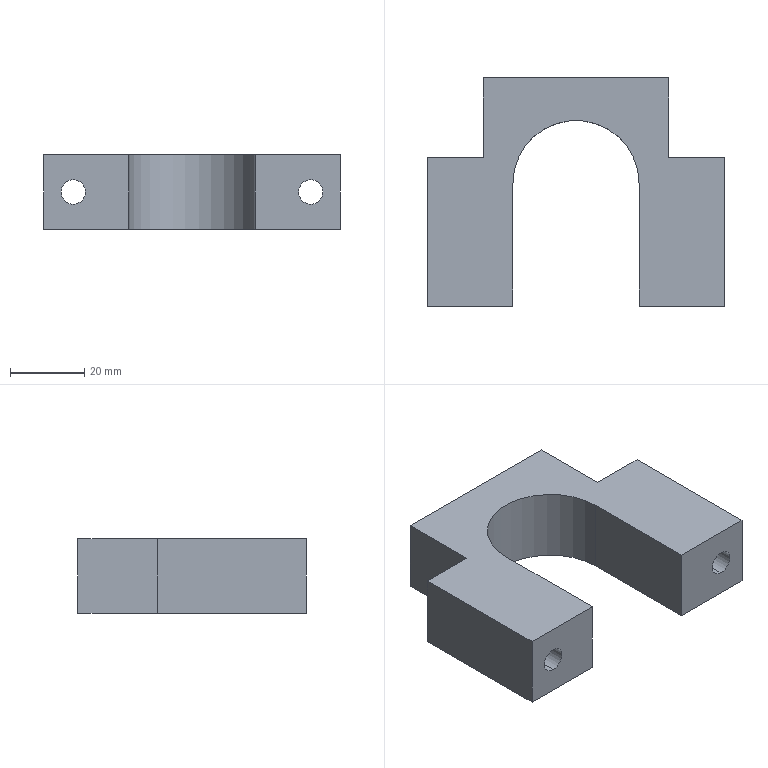Part | STEP file | 866-BDO024-93-12A | 1 solid | 24 faces | box 80 x 61.5 x 20 mm | volume 50514 mm3 | plane 15 | cylinder 9 | commonest cylinder face diameters 6.6 x4 11 x4 34 x1
STEP:
#1=CARTESIAN_POINT('',(-32.,34.,-5.5));
#2=VERTEX_POINT('',#1);
#3=CARTESIAN_POINT('',(-32.,34.,5.5));
#4=VERTEX_POINT('',#3);
#5=CARTESIAN_POINT('',(-32.,34.,0.));
#6=DIRECTION('',(0.,1.,0.));
#7=DIRECTION('',(0.,0.,1.));
#8=AXIS2_PLACEMENT_3D('',#5,#6,#7);
#9=CIRCLE('',#8,5.5);
#10=EDGE_CURVE('',#2,#4,#9,.T.);
#11=ORIENTED_EDGE('',*,*,#10,.F.);
#12=CARTESIAN_POINT('',(-32.,40.,-5.5));
#13=VERTEX_POINT('',#12);
#14=CARTESIAN_POINT('',(-32.,40.,-5.5));
#15=DIRECTION('',(0.,1.,0.));
#16=VECTOR('',#15,1000.);
#17=LINE('',#14,#16);
#18=EDGE_CURVE('',#2,#13,#17,.T.);
#19=ORIENTED_EDGE('',*,*,#18,.T.);
#20=CARTESIAN_POINT('',(-32.,40.,5.5));
#21=VERTEX_POINT('',#20);
#22=CARTESIAN_POINT('',(-32.,40.,0.));
#23=DIRECTION('',(0.,1.,0.));
#24=DIRECTION('',(0.,0.,1.));
#25=AXIS2_PLACEMENT_3D('',#22,#23,#24);
#26=CIRCLE('',#25,5.5);
#27=EDGE_CURVE('',#13,#21,#26,.T.);
#28=ORIENTED_EDGE('',*,*,#27,.T.);
#29=CARTESIAN_POINT('',(-32.,40.,5.5));
#30=DIRECTION('',(0.,1.,0.));
#31=VECTOR('',#30,1000.);
#32=LINE('',#29,#31);
#33=EDGE_CURVE('',#4,#21,#32,.T.);
#34=ORIENTED_EDGE('',*,*,#33,.F.);
#35=EDGE_LOOP('',(#11,#19,#28,#34));
#36=FACE_OUTER_BOUND('',#35,.T.);
#37=CARTESIAN_POINT('',(-32.,40.,0.));
#38=DIRECTION('',(0.,1.,0.));
#39=DIRECTION('',(0.,0.,1.));
#40=AXIS2_PLACEMENT_3D('',#37,#38,#39);
#41=CYLINDRICAL_SURFACE('',#40,5.5);
#42=ADVANCED_FACE('',(#36),#41,.F.);
#43=CARTESIAN_POINT('',(32.,34.,-5.5));
#44=VERTEX_POINT('',#43);
#45=CARTESIAN_POINT('',(32.,34.,5.5));
#46=VERTEX_POINT('',#45);
#47=CARTESIAN_POINT('',(32.,34.,0.));
#48=DIRECTION('',(0.,1.,0.));
#49=DIRECTION('',(0.,0.,1.));
#50=AXIS2_PLACEMENT_3D('',#47,#48,#49);
#51=CIRCLE('',#50,5.5);
#52=EDGE_CURVE('',#44,#46,#51,.T.);
#53=ORIENTED_EDGE('',*,*,#52,.F.);
#54=CARTESIAN_POINT('',(32.,40.,-5.5));
#55=VERTEX_POINT('',#54);
#56=CARTESIAN_POINT('',(32.,40.,-5.5));
#57=DIRECTION('',(0.,1.,0.));
#58=VECTOR('',#57,1000.);
#59=LINE('',#56,#58);
#60=EDGE_CURVE('',#44,#55,#59,.T.);
#61=ORIENTED_EDGE('',*,*,#60,.T.);
#62=CARTESIAN_POINT('',(32.,40.,5.5));
#63=VERTEX_POINT('',#62);
#64=CARTESIAN_POINT('',(32.,40.,0.));
#65=DIRECTION('',(0.,1.,0.));
#66=DIRECTION('',(0.,0.,1.));
#67=AXIS2_PLACEMENT_3D('',#64,#65,#66);
#68=CIRCLE('',#67,5.5);
#69=EDGE_CURVE('',#55,#63,#68,.T.);
#70=ORIENTED_EDGE('',*,*,#69,.T.);
#71=CARTESIAN_POINT('',(32.,40.,5.5));
#72=DIRECTION('',(0.,1.,0.));
#73=VECTOR('',#72,1000.);
#74=LINE('',#71,#73);
#75=EDGE_CURVE('',#46,#63,#74,.T.);
#76=ORIENTED_EDGE('',*,*,#75,.F.);
#77=EDGE_LOOP('',(#53,#61,#70,#76));
#78=FACE_OUTER_BOUND('',#77,.T.);
#79=CARTESIAN_POINT('',(32.,40.,0.));
#80=DIRECTION('',(0.,1.,0.));
#81=DIRECTION('',(0.,0.,1.));
#82=AXIS2_PLACEMENT_3D('',#79,#80,#81);
#83=CYLINDRICAL_SURFACE('',#82,5.5);
#84=ADVANCED_FACE('',(#78),#83,.F.);
#85=CARTESIAN_POINT('',(32.,0.,3.3));
#86=VERTEX_POINT('',#85);
#87=CARTESIAN_POINT('',(32.,0.,-3.3));
#88=VERTEX_POINT('',#87);
#89=CARTESIAN_POINT('',(32.,0.,0.));
#90=DIRECTION('',(0.,-1.,0.));
#91=DIRECTION('',(0.,0.,1.));
#92=AXIS2_PLACEMENT_3D('',#89,#90,#91);
#93=CIRCLE('',#92,3.3);
#94=EDGE_CURVE('',#86,#88,#93,.T.);
#95=ORIENTED_EDGE('',*,*,#94,.T.);
#96=CARTESIAN_POINT('',(32.,34.,-3.3));
#97=VERTEX_POINT('',#96);
#98=CARTESIAN_POINT('',(32.,40.,-3.3));
#99=DIRECTION('',(0.,1.,0.));
#100=VECTOR('',#99,1000.);
#101=LINE('',#98,#100);
#102=EDGE_CURVE('',#88,#97,#101,.T.);
#103=ORIENTED_EDGE('',*,*,#102,.T.);
#104=CARTESIAN_POINT('',(32.,34.,3.3));
#105=VERTEX_POINT('',#104);
#106=CARTESIAN_POINT('',(32.,34.,0.));
#107=DIRECTION('',(0.,-1.,0.));
#108=DIRECTION('',(0.,0.,1.));
#109=AXIS2_PLACEMENT_3D('',#106,#107,#108);
#110=CIRCLE('',#109,3.3);
#111=EDGE_CURVE('',#105,#97,#110,.T.);
#112=ORIENTED_EDGE('',*,*,#111,.F.);
#113=CARTESIAN_POINT('',(32.,40.,3.3));
#114=DIRECTION('',(0.,1.,0.));
#115=VECTOR('',#114,1000.);
#116=LINE('',#113,#115);
#117=EDGE_CURVE('',#86,#105,#116,.T.);
#118=ORIENTED_EDGE('',*,*,#117,.F.);
#119=EDGE_LOOP('',(#95,#103,#112,#118));
#120=FACE_OUTER_BOUND('',#119,.T.);
#121=CARTESIAN_POINT('',(32.,40.,0.));
#122=DIRECTION('',(0.,1.,0.));
#123=DIRECTION('',(0.,0.,1.));
#124=AXIS2_PLACEMENT_3D('',#121,#122,#123);
#125=CYLINDRICAL_SURFACE('',#124,3.3);
#126=ADVANCED_FACE('',(#120),#125,.F.);
#127=CARTESIAN_POINT('',(-32.,0.,3.3));
#128=VERTEX_POINT('',#127);
#129=CARTESIAN_POINT('',(-32.,0.,-3.3));
#130=VERTEX_POINT('',#129);
#131=CARTESIAN_POINT('',(-32.,0.,0.));
#132=DIRECTION('',(0.,-1.,0.));
#133=DIRECTION('',(0.,0.,1.));
#134=AXIS2_PLACEMENT_3D('',#131,#132,#133);
#135=CIRCLE('',#134,3.3);
#136=EDGE_CURVE('',#128,#130,#135,.T.);
#137=ORIENTED_EDGE('',*,*,#136,.T.);
#138=CARTESIAN_POINT('',(-32.,34.,-3.3));
#139=VERTEX_POINT('',#138);
#140=CARTESIAN_POINT('',(-32.,40.,-3.3));
#141=DIRECTION('',(0.,1.,0.));
#142=VECTOR('',#141,1000.);
#143=LINE('',#140,#142);
#144=EDGE_CURVE('',#130,#139,#143,.T.);
#145=ORIENTED_EDGE('',*,*,#144,.T.);
#146=CARTESIAN_POINT('',(-32.,34.,3.3));
#147=VERTEX_POINT('',#146);
#148=CARTESIAN_POINT('',(-32.,34.,0.));
#149=DIRECTION('',(0.,-1.,0.));
#150=DIRECTION('',(0.,0.,1.));
#151=AXIS2_PLACEMENT_3D('',#148,#149,#150);
#152=CIRCLE('',#151,3.3);
#153=EDGE_CURVE('',#147,#139,#152,.T.);
#154=ORIENTED_EDGE('',*,*,#153,.F.);
#155=CARTESIAN_POINT('',(-32.,40.,3.3));
#156=DIRECTION('',(0.,1.,0.));
#157=VECTOR('',#156,1000.);
#158=LINE('',#155,#157);
#159=EDGE_CURVE('',#128,#147,#158,.T.);
#160=ORIENTED_EDGE('',*,*,#159,.F.);
#161=EDGE_LOOP('',(#137,#145,#154,#160));
#162=FACE_OUTER_BOUND('',#161,.T.);
#163=CARTESIAN_POINT('',(-32.,40.,0.));
#164=DIRECTION('',(0.,1.,0.));
#165=DIRECTION('',(0.,0.,1.));
#166=AXIS2_PLACEMENT_3D('',#163,#164,#165);
#167=CYLINDRICAL_SURFACE('',#166,3.3);
#168=ADVANCED_FACE('',(#162),#167,.F.);
#169=CARTESIAN_POINT('',(-25.,61.5,10.));
#170=VERTEX_POINT('',#169);
#171=CARTESIAN_POINT('',(-25.,40.,10.));
#172=VERTEX_POINT('',#171);
#173=CARTESIAN_POINT('',(-25.,33.,10.));
#174=DIRECTION('',(0.,-1.,0.));
#175=VECTOR('',#174,1000.);
#176=LINE('',#173,#175);
#177=EDGE_CURVE('',#170,#172,#176,.T.);
#178=ORIENTED_EDGE('',*,*,#177,.T.);
#179=CARTESIAN_POINT('',(-40.,40.,10.));
#180=VERTEX_POINT('',#179);
#181=CARTESIAN_POINT('',(0.,40.,10.));
#182=DIRECTION('',(-1.,0.,0.));
#183=VECTOR('',#182,1000.);
#184=LINE('',#181,#183);
#185=EDGE_CURVE('',#172,#180,#184,.T.);
#186=ORIENTED_EDGE('',*,*,#185,.T.);
#187=CARTESIAN_POINT('',(-40.,0.,10.));
#188=VERTEX_POINT('',#187);
#189=CARTESIAN_POINT('',(-40.,33.,10.));
#190=DIRECTION('',(0.,-1.,0.));
#191=VECTOR('',#190,1000.);
#192=LINE('',#189,#191);
#193=EDGE_CURVE('',#180,#188,#192,.T.);
#194=ORIENTED_EDGE('',*,*,#193,.T.);
#195=CARTESIAN_POINT('',(-17.,0.,10.));
#196=VERTEX_POINT('',#195);
#197=CARTESIAN_POINT('',(0.,0.,10.));
#198=DIRECTION('',(1.,0.,0.));
#199=VECTOR('',#198,1000.);
#200=LINE('',#197,#199);
#201=EDGE_CURVE('',#188,#196,#200,.T.);
#202=ORIENTED_EDGE('',*,*,#201,.T.);
#203=CARTESIAN_POINT('',(-17.,33.,10.));
#204=VERTEX_POINT('',#203);
#205=CARTESIAN_POINT('',(-17.,33.,10.));
#206=DIRECTION('',(0.,1.,0.));
#207=VECTOR('',#206,1000.);
#208=LINE('',#205,#207);
#209=EDGE_CURVE('',#196,#204,#208,.T.);
#210=ORIENTED_EDGE('',*,*,#209,.T.);
#211=CARTESIAN_POINT('',(17.,33.,10.));
#212=VERTEX_POINT('',#211);
#213=CARTESIAN_POINT('',(0.,33.,10.));
#214=DIRECTION('',(0.,0.,-1.));
#215=DIRECTION('',(-1.,0.,0.));
#216=AXIS2_PLACEMENT_3D('',#213,#214,#215);
#217=CIRCLE('',#216,17.);
#218=EDGE_CURVE('',#204,#212,#217,.T.);
#219=ORIENTED_EDGE('',*,*,#218,.T.);
#220=CARTESIAN_POINT('',(17.,0.,10.));
#221=VERTEX_POINT('',#220);
#222=CARTESIAN_POINT('',(17.,33.,10.));
#223=DIRECTION('',(0.,-1.,0.));
#224=VECTOR('',#223,1000.);
#225=LINE('',#222,#224);
#226=EDGE_CURVE('',#212,#221,#225,.T.);
#227=ORIENTED_EDGE('',*,*,#226,.T.);
#228=CARTESIAN_POINT('',(40.,0.,10.));
#229=VERTEX_POINT('',#228);
#230=CARTESIAN_POINT('',(0.,0.,10.));
#231=DIRECTION('',(1.,0.,0.));
#232=VECTOR('',#231,1000.);
#233=LINE('',#230,#232);
#234=EDGE_CURVE('',#221,#229,#233,.T.);
#235=ORIENTED_EDGE('',*,*,#234,.T.);
#236=CARTESIAN_POINT('',(40.,40.,10.));
#237=VERTEX_POINT('',#236);
#238=CARTESIAN_POINT('',(40.,33.,10.));
#239=DIRECTION('',(0.,1.,0.));
#240=VECTOR('',#239,1000.);
#241=LINE('',#238,#240);
#242=EDGE_CURVE('',#229,#237,#241,.T.);
#243=ORIENTED_EDGE('',*,*,#242,.T.);
#244=CARTESIAN_POINT('',(25.,40.,10.));
#245=VERTEX_POINT('',#244);
#246=CARTESIAN_POINT('',(0.,40.,10.));
#247=DIRECTION('',(-1.,0.,0.));
#248=VECTOR('',#247,1000.);
#249=LINE('',#246,#248);
#250=EDGE_CURVE('',#237,#245,#249,.T.);
#251=ORIENTED_EDGE('',*,*,#250,.T.);
#252=CARTESIAN_POINT('',(25.,61.5,10.));
#253=VERTEX_POINT('',#252);
#254=CARTESIAN_POINT('',(25.,33.,10.));
#255=DIRECTION('',(0.,1.,0.));
#256=VECTOR('',#255,1000.);
#257=LINE('',#254,#256);
#258=EDGE_CURVE('',#245,#253,#257,.T.);
#259=ORIENTED_EDGE('',*,*,#258,.T.);
#260=CARTESIAN_POINT('',(0.,61.5,10.));
#261=DIRECTION('',(-1.,0.,0.));
#262=VECTOR('',#261,1000.);
#263=LINE('',#260,#262);
#264=EDGE_CURVE('',#253,#170,#263,.T.);
#265=ORIENTED_EDGE('',*,*,#264,.T.);
#266=EDGE_LOOP('',(#178,#186,#194,#202,#210,#219,#227,#235,#243,#251,#259,#265));
#267=FACE_OUTER_BOUND('',#266,.T.);
#268=CARTESIAN_POINT('',(0.,33.,10.));
#269=DIRECTION('',(0.,0.,1.));
#270=DIRECTION('',(1.,0.,0.));
#271=AXIS2_PLACEMENT_3D('',#268,#269,#270);
#272=PLANE('',#271);
#273=ADVANCED_FACE('',(#267),#272,.T.);
#274=CARTESIAN_POINT('',(-40.,40.,-10.));
#275=VERTEX_POINT('',#274);
#276=CARTESIAN_POINT('',(-40.,40.,10.));
#277=DIRECTION('',(0.,0.,-1.));
#278=VECTOR('',#277,1000.);
#279=LINE('',#276,#278);
#280=EDGE_CURVE('',#180,#275,#279,.T.);
#281=ORIENTED_EDGE('',*,*,#280,.F.);
#282=ORIENTED_EDGE('',*,*,#185,.F.);
#283=CARTESIAN_POINT('',(-25.,40.,-10.));
#284=VERTEX_POINT('',#283);
#285=CARTESIAN_POINT('',(-25.,40.,10.));
#286=DIRECTION('',(0.,0.,1.));
#287=VECTOR('',#286,1000.);
#288=LINE('',#285,#287);
#289=EDGE_CURVE('',#284,#172,#288,.T.);
#290=ORIENTED_EDGE('',*,*,#289,.F.);
#291=CARTESIAN_POINT('',(-40.,40.,-10.));
#292=DIRECTION('',(1.,0.,0.));
#293=VECTOR('',#292,1000.);
#294=LINE('',#291,#293);
#295=EDGE_CURVE('',#275,#284,#294,.T.);
#296=ORIENTED_EDGE('',*,*,#295,.F.);
#297=EDGE_LOOP('',(#281,#282,#290,#296));
#298=FACE_OUTER_BOUND('',#297,.T.);
#299=CARTESIAN_POINT('',(-32.,40.,0.));
#300=DIRECTION('',(0.,1.,0.));
#301=DIRECTION('',(0.,0.,1.));
#302=AXIS2_PLACEMENT_3D('',#299,#300,#301);
#303=CIRCLE('',#302,5.5);
#304=EDGE_CURVE('',#21,#13,#303,.T.);
#305=ORIENTED_EDGE('',*,*,#304,.F.);
#306=ORIENTED_EDGE('',*,*,#27,.F.);
#307=EDGE_LOOP('',(#305,#306));
#308=FACE_BOUND('',#307,.T.);
#309=CARTESIAN_POINT('',(-40.,40.,10.));
#310=DIRECTION('',(0.,-1.,0.));
#311=DIRECTION('',(0.,0.,-1.));
#312=AXIS2_PLACEMENT_3D('',#309,#310,#311);
#313=PLANE('',#312);
#314=ADVANCED_FACE('',(#298,#308),#313,.F.);
#315=ORIENTED_EDGE('',*,*,#289,.T.);
#316=ORIENTED_EDGE('',*,*,#177,.F.);
#317=CARTESIAN_POINT('',(-25.,61.5,-10.));
#318=VERTEX_POINT('',#317);
#319=CARTESIAN_POINT('',(-25.,61.5,10.));
#320=DIRECTION('',(0.,0.,1.));
#321=VECTOR('',#320,1000.);
#322=LINE('',#319,#321);
#323=EDGE_CURVE('',#318,#170,#322,.T.);
#324=ORIENTED_EDGE('',*,*,#323,.F.);
#325=CARTESIAN_POINT('',(-25.,40.,-10.));
#326=DIRECTION('',(0.,1.,0.));
#327=VECTOR('',#326,1000.);
#328=LINE('',#325,#327);
#329=EDGE_CURVE('',#284,#318,#328,.T.);
#330=ORIENTED_EDGE('',*,*,#329,.F.);
#331=EDGE_LOOP('',(#315,#316,#324,#330));
#332=FACE_OUTER_BOUND('',#331,.T.);
#333=CARTESIAN_POINT('',(-25.,40.,10.));
#334=DIRECTION('',(1.,0.,0.));
#335=DIRECTION('',(0.,1.,0.));
#336=AXIS2_PLACEMENT_3D('',#333,#334,#335);
#337=PLANE('',#336);
#338=ADVANCED_FACE('',(#332),#337,.F.);
#339=ORIENTED_EDGE('',*,*,#323,.T.);
#340=ORIENTED_EDGE('',*,*,#264,.F.);
#341=CARTESIAN_POINT('',(25.,61.5,-10.));
#342=VERTEX_POINT('',#341);
#343=CARTESIAN_POINT('',(25.,61.5,10.));
#344=DIRECTION('',(0.,0.,1.));
#345=VECTOR('',#344,1000.);
#346=LINE('',#343,#345);
#347=EDGE_CURVE('',#342,#253,#346,.T.);
#348=ORIENTED_EDGE('',*,*,#347,.F.);
#349=CARTESIAN_POINT('',(-25.,61.5,-10.));
#350=DIRECTION('',(1.,0.,0.));
#351=VECTOR('',#350,1000.);
#352=LINE('',#349,#351);
#353=EDGE_CURVE('',#318,#342,#352,.T.);
#354=ORIENTED_EDGE('',*,*,#353,.F.);
#355=EDGE_LOOP('',(#339,#340,#348,#354));
#356=FACE_OUTER_BOUND('',#355,.T.);
#357=CARTESIAN_POINT('',(-25.,61.5,10.));
#358=DIRECTION('',(0.,-1.,0.));
#359=DIRECTION('',(0.,0.,-1.));
#360=AXIS2_PLACEMENT_3D('',#357,#358,#359);
#361=PLANE('',#360);
#362=ADVANCED_FACE('',(#356),#361,.F.);
#363=ORIENTED_EDGE('',*,*,#347,.T.);
#364=ORIENTED_EDGE('',*,*,#258,.F.);
#365=CARTESIAN_POINT('',(25.,40.,-10.));
#366=VERTEX_POINT('',#365);
#367=CARTESIAN_POINT('',(25.,40.,10.));
#368=DIRECTION('',(0.,0.,1.));
#369=VECTOR('',#368,1000.);
#370=LINE('',#367,#369);
#371=EDGE_CURVE('',#366,#245,#370,.T.);
#372=ORIENTED_EDGE('',*,*,#371,.F.);
#373=CARTESIAN_POINT('',(25.,61.5,-10.));
#374=DIRECTION('',(0.,-1.,0.));
#375=VECTOR('',#374,1000.);
#376=LINE('',#373,#375);
#377=EDGE_CURVE('',#342,#366,#376,.T.);
#378=ORIENTED_EDGE('',*,*,#377,.F.);
#379=EDGE_LOOP('',(#363,#364,#372,#378));
#380=FACE_OUTER_BOUND('',#379,.T.);
#381=CARTESIAN_POINT('',(25.,61.5,10.));
#382=DIRECTION('',(-1.,0.,0.));
#383=DIRECTION('',(0.,-1.,0.));
#384=AXIS2_PLACEMENT_3D('',#381,#382,#383);
#385=PLANE('',#384);
#386=ADVANCED_FACE('',(#380),#385,.F.);
#387=ORIENTED_EDGE('',*,*,#371,.T.);
#388=ORIENTED_EDGE('',*,*,#250,.F.);
#389=CARTESIAN_POINT('',(40.,40.,-10.));
#390=VERTEX_POINT('',#389);
#391=CARTESIAN_POINT('',(40.,40.,10.));
#392=DIRECTION('',(0.,0.,1.));
#393=VECTOR('',#392,1000.);
#394=LINE('',#391,#393);
#395=EDGE_CURVE('',#390,#237,#394,.T.);
#396=ORIENTED_EDGE('',*,*,#395,.F.);
#397=CARTESIAN_POINT('',(25.,40.,-10.));
#398=DIRECTION('',(1.,0.,0.));
#399=VECTOR('',#398,1000.);
#400=LINE('',#397,#399);
#401=EDGE_CURVE('',#366,#390,#400,.T.);
#402=ORIENTED_EDGE('',*,*,#401,.F.);
#403=EDGE_LOOP('',(#387,#388,#396,#402));
#404=FACE_OUTER_BOUND('',#403,.T.);
#405=CARTESIAN_POINT('',(32.,40.,0.));
#406=DIRECTION('',(0.,1.,0.));
#407=DIRECTION('',(0.,0.,1.));
#408=AXIS2_PLACEMENT_3D('',#405,#406,#407);
#409=CIRCLE('',#408,5.5);
#410=EDGE_CURVE('',#63,#55,#409,.T.);
#411=ORIENTED_EDGE('',*,*,#410,.F.);
#412=ORIENTED_EDGE('',*,*,#69,.F.);
#413=EDGE_LOOP('',(#411,#412));
#414=FACE_BOUND('',#413,.T.);
#415=CARTESIAN_POINT('',(25.,40.,10.));
#416=DIRECTION('',(0.,-1.,0.));
#417=DIRECTION('',(0.,0.,-1.));
#418=AXIS2_PLACEMENT_3D('',#415,#416,#417);
#419=PLANE('',#418);
#420=ADVANCED_FACE('',(#404,#414),#419,.F.);
#421=ORIENTED_EDGE('',*,*,#395,.T.);
#422=ORIENTED_EDGE('',*,*,#242,.F.);
#423=CARTESIAN_POINT('',(40.,0.,-10.));
#424=VERTEX_POINT('',#423);
#425=CARTESIAN_POINT('',(40.,0.,10.));
#426=DIRECTION('',(0.,0.,1.));
#427=VECTOR('',#426,1000.);
#428=LINE('',#425,#427);
#429=EDGE_CURVE('',#424,#229,#428,.T.);
#430=ORIENTED_EDGE('',*,*,#429,.F.);
#431=CARTESIAN_POINT('',(40.,0.,-10.));
#432=DIRECTION('',(0.,-1.,0.));
#433=VECTOR('',#432,1000.);
#434=LINE('',#431,#433);
#435=EDGE_CURVE('',#390,#424,#434,.T.);
#436=ORIENTED_EDGE('',*,*,#435,.F.);
#437=EDGE_LOOP('',(#421,#422,#430,#436));
#438=FACE_OUTER_BOUND('',#437,.T.);
#439=CARTESIAN_POINT('',(40.,0.,10.));
#440=DIRECTION('',(-1.,0.,0.));
#441=DIRECTION('',(0.,0.,1.));
#442=AXIS2_PLACEMENT_3D('',#439,#440,#441);
#443=PLANE('',#442);
#444=ADVANCED_FACE('',(#438),#443,.F.);
#445=ORIENTED_EDGE('',*,*,#429,.T.);
#446=ORIENTED_EDGE('',*,*,#234,.F.);
#447=CARTESIAN_POINT('',(17.,0.,-10.));
#448=VERTEX_POINT('',#447);
#449=CARTESIAN_POINT('',(17.,0.,10.));
#450=DIRECTION('',(0.,0.,1.));
#451=VECTOR('',#450,1000.);
#452=LINE('',#449,#451);
#453=EDGE_CURVE('',#448,#221,#452,.T.);
#454=ORIENTED_EDGE('',*,*,#453,.F.);
#455=CARTESIAN_POINT('',(17.,0.,-10.));
#456=DIRECTION('',(-1.,0.,0.));
#457=VECTOR('',#456,1000.);
#458=LINE('',#455,#457);
#459=EDGE_CURVE('',#424,#448,#458,.T.);
#460=ORIENTED_EDGE('',*,*,#459,.F.);
#461=EDGE_LOOP('',(#445,#446,#454,#460));
#462=FACE_OUTER_BOUND('',#461,.T.);
#463=ORIENTED_EDGE('',*,*,#94,.F.);
#464=CARTESIAN_POINT('',(32.,0.,0.));
#465=DIRECTION('',(0.,-1.,0.));
#466=DIRECTION('',(0.,0.,1.));
#467=AXIS2_PLACEMENT_3D('',#464,#465,#466);
#468=CIRCLE('',#467,3.3);
#469=EDGE_CURVE('',#88,#86,#468,.T.);
#470=ORIENTED_EDGE('',*,*,#469,.F.);
#471=EDGE_LOOP('',(#463,#470));
#472=FACE_BOUND('',#471,.T.);
#473=CARTESIAN_POINT('',(17.,0.,10.));
#474=DIRECTION('',(0.,1.,0.));
#475=DIRECTION('',(0.,0.,1.));
#476=AXIS2_PLACEMENT_3D('',#473,#474,#475);
#477=PLANE('',#476);
#478=ADVANCED_FACE('',(#462,#472),#477,.F.);
#479=ORIENTED_EDGE('',*,*,#453,.T.);
#480=ORIENTED_EDGE('',*,*,#226,.F.);
#481=CARTESIAN_POINT('',(17.,33.,-10.));
#482=VERTEX_POINT('',#481);
#483=CARTESIAN_POINT('',(17.,33.,10.));
#484=DIRECTION('',(0.,0.,1.));
#485=VECTOR('',#484,1000.);
#486=LINE('',#483,#485);
#487=EDGE_CURVE('',#482,#212,#486,.T.);
#488=ORIENTED_EDGE('',*,*,#487,.F.);
#489=CARTESIAN_POINT('',(17.,33.,-10.));
#490=DIRECTION('',(0.,1.,0.));
#491=VECTOR('',#490,1000.);
#492=LINE('',#489,#491);
#493=EDGE_CURVE('',#448,#482,#492,.T.);
#494=ORIENTED_EDGE('',*,*,#493,.F.);
#495=EDGE_LOOP('',(#479,#480,#488,#494));
#496=FACE_OUTER_BOUND('',#495,.T.);
#497=CARTESIAN_POINT('',(17.,33.,10.));
#498=DIRECTION('',(1.,0.,0.));
#499=DIRECTION('',(0.,1.,0.));
#500=AXIS2_PLACEMENT_3D('',#497,#498,#499);
#501=PLANE('',#500);
#502=ADVANCED_FACE('',(#496),#501,.F.);
#503=ORIENTED_EDGE('',*,*,#487,.T.);
#504=ORIENTED_EDGE('',*,*,#218,.F.);
#505=CARTESIAN_POINT('',(-17.,33.,-10.));
#506=VERTEX_POINT('',#505);
#507=CARTESIAN_POINT('',(-17.,33.,10.));
#508=DIRECTION('',(0.,0.,1.));
#509=VECTOR('',#508,1000.);
#510=LINE('',#507,#509);
#511=EDGE_CURVE('',#506,#204,#510,.T.);
#512=ORIENTED_EDGE('',*,*,#511,.F.);
#513=CARTESIAN_POINT('',(0.,33.,-10.));
#514=DIRECTION('',(0.,0.,1.));
#515=DIRECTION('',(-1.,0.,0.));
#516=AXIS2_PLACEMENT_3D('',#513,#514,#515);
#517=CIRCLE('',#516,17.);
#518=EDGE_CURVE('',#482,#506,#517,.T.);
#519=ORIENTED_EDGE('',*,*,#518,.F.);
#520=EDGE_LOOP('',(#503,#504,#512,#519));
#521=FACE_OUTER_BOUND('',#520,.T.);
#522=CARTESIAN_POINT('',(0.,33.,10.));
#523=DIRECTION('',(0.,0.,-1.));
#524=DIRECTION('',(-1.,0.,0.));
#525=AXIS2_PLACEMENT_3D('',#522,#523,#524);
#526=CYLINDRICAL_SURFACE('',#525,17.);
#527=ADVANCED_FACE('',(#521),#526,.F.);
#528=ORIENTED_EDGE('',*,*,#511,.T.);
#529=ORIENTED_EDGE('',*,*,#209,.F.);
#530=CARTESIAN_POINT('',(-17.,0.,-10.));
#531=VERTEX_POINT('',#530);
#532=CARTESIAN_POINT('',(-17.,0.,10.));
#533=DIRECTION('',(0.,0.,1.));
#534=VECTOR('',#533,1000.);
#535=LINE('',#532,#534);
#536=EDGE_CURVE('',#531,#196,#535,.T.);
#537=ORIENTED_EDGE('',*,*,#536,.F.);
#538=CARTESIAN_POINT('',(-17.,33.,-10.));
#539=DIRECTION('',(0.,-1.,0.));
#540=VECTOR('',#539,1000.);
#541=LINE('',#538,#540);
#542=EDGE_CURVE('',#506,#531,#541,.T.);
#543=ORIENTED_EDGE('',*,*,#542,.F.);
#544=EDGE_LOOP('',(#528,#529,#537,#543));
#545=FACE_OUTER_BOUND('',#544,.T.);
#546=CARTESIAN_POINT('',(-17.,33.,10.));
#547=DIRECTION('',(-1.,0.,0.));
#548=DIRECTION('',(0.,-1.,0.));
#549=AXIS2_PLACEMENT_3D('',#546,#547,#548);
#550=PLANE('',#549);
#551=ADVANCED_FACE('',(#545),#550,.F.);
#552=ORIENTED_EDGE('',*,*,#536,.T.);
#553=ORIENTED_EDGE('',*,*,#201,.F.);
#554=CARTESIAN_POINT('',(-40.,0.,-10.));
#555=VERTEX_POINT('',#554);
#556=CARTESIAN_POINT('',(-40.,0.,10.));
#557=DIRECTION('',(0.,0.,1.));
#558=VECTOR('',#557,1000.);
#559=LINE('',#556,#558);
#560=EDGE_CURVE('',#555,#188,#559,.T.);
#561=ORIENTED_EDGE('',*,*,#560,.F.);
#562=CARTESIAN_POINT('',(-40.,0.,-10.));
#563=DIRECTION('',(-1.,0.,0.));
#564=VECTOR('',#563,1000.);
#565=LINE('',#562,#564);
#566=EDGE_CURVE('',#531,#555,#565,.T.);
#567=ORIENTED_EDGE('',*,*,#566,.F.);
#568=EDGE_LOOP('',(#552,#553,#561,#567));
#569=FACE_OUTER_BOUND('',#568,.T.);
#570=ORIENTED_EDGE('',*,*,#136,.F.);
#571=CARTESIAN_POINT('',(-32.,0.,0.));
#572=DIRECTION('',(0.,-1.,0.));
#573=DIRECTION('',(0.,0.,1.));
#574=AXIS2_PLACEMENT_3D('',#571,#572,#573);
#575=CIRCLE('',#574,3.3);
#576=EDGE_CURVE('',#130,#128,#575,.T.);
#577=ORIENTED_EDGE('',*,*,#576,.F.);
#578=EDGE_LOOP('',(#570,#577));
#579=FACE_BOUND('',#578,.T.);
#580=CARTESIAN_POINT('',(-40.,0.,10.));
#581=DIRECTION('',(0.,1.,0.));
#582=DIRECTION('',(0.,0.,1.));
#583=AXIS2_PLACEMENT_3D('',#580,#581,#582);
#584=PLANE('',#583);
#585=ADVANCED_FACE('',(#569,#579),#584,.F.);
#586=ORIENTED_EDGE('',*,*,#560,.T.);
#587=ORIENTED_EDGE('',*,*,#193,.F.);
#588=ORIENTED_EDGE('',*,*,#280,.T.);
#589=CARTESIAN_POINT('',(-40.,0.,-10.));
#590=DIRECTION('',(0.,1.,0.));
#591=VECTOR('',#590,1000.);
#592=LINE('',#589,#591);
#593=EDGE_CURVE('',#555,#275,#592,.T.);
#594=ORIENTED_EDGE('',*,*,#593,.F.);
#595=EDGE_LOOP('',(#586,#587,#588,#594));
#596=FACE_OUTER_BOUND('',#595,.T.);
#597=CARTESIAN_POINT('',(-40.,0.,10.));
#598=DIRECTION('',(1.,0.,0.));
#599=DIRECTION('',(0.,0.,-1.));
#600=AXIS2_PLACEMENT_3D('',#597,#598,#599);
#601=PLANE('',#600);
#602=ADVANCED_FACE('',(#596),#601,.F.);
#603=ORIENTED_EDGE('',*,*,#295,.T.);
#604=ORIENTED_EDGE('',*,*,#329,.T.);
#605=ORIENTED_EDGE('',*,*,#353,.T.);
#606=ORIENTED_EDGE('',*,*,#377,.T.);
#607=ORIENTED_EDGE('',*,*,#401,.T.);
#608=ORIENTED_EDGE('',*,*,#435,.T.);
#609=ORIENTED_EDGE('',*,*,#459,.T.);
#610=ORIENTED_EDGE('',*,*,#493,.T.);
#611=ORIENTED_EDGE('',*,*,#518,.T.);
#612=ORIENTED_EDGE('',*,*,#542,.T.);
#613=ORIENTED_EDGE('',*,*,#566,.T.);
#614=ORIENTED_EDGE('',*,*,#593,.T.);
#615=EDGE_LOOP('',(#603,#604,#605,#606,#607,#608,#609,#610,#611,#612,#613,#614));
#616=FACE_OUTER_BOUND('',#615,.T.);
#617=CARTESIAN_POINT('',(0.,33.,-10.));
#618=DIRECTION('',(0.,0.,1.));
#619=DIRECTION('',(1.,0.,0.));
#620=AXIS2_PLACEMENT_3D('',#617,#618,#619);
#621=PLANE('',#620);
#622=ADVANCED_FACE('',(#616),#621,.F.);
#623=ORIENTED_EDGE('',*,*,#18,.F.);
#624=CARTESIAN_POINT('',(-32.,34.,0.));
#625=DIRECTION('',(0.,1.,0.));
#626=DIRECTION('',(0.,0.,1.));
#627=AXIS2_PLACEMENT_3D('',#624,#625,#626);
#628=CIRCLE('',#627,5.5);
#629=EDGE_CURVE('',#4,#2,#628,.T.);
#630=ORIENTED_EDGE('',*,*,#629,.F.);
#631=ORIENTED_EDGE('',*,*,#33,.T.);
#632=ORIENTED_EDGE('',*,*,#304,.T.);
#633=EDGE_LOOP('',(#623,#630,#631,#632));
#634=FACE_OUTER_BOUND('',#633,.T.);
#635=CARTESIAN_POINT('',(-32.,40.,0.));
#636=DIRECTION('',(0.,1.,0.));
#637=DIRECTION('',(0.,0.,1.));
#638=AXIS2_PLACEMENT_3D('',#635,#636,#637);
#639=CYLINDRICAL_SURFACE('',#638,5.5);
#640=ADVANCED_FACE('',(#634),#639,.F.);
#641=ORIENTED_EDGE('',*,*,#60,.F.);
#642=CARTESIAN_POINT('',(32.,34.,0.));
#643=DIRECTION('',(0.,1.,0.));
#644=DIRECTION('',(0.,0.,1.));
#645=AXIS2_PLACEMENT_3D('',#642,#643,#644);
#646=CIRCLE('',#645,5.5);
#647=EDGE_CURVE('',#46,#44,#646,.T.);
#648=ORIENTED_EDGE('',*,*,#647,.F.);
#649=ORIENTED_EDGE('',*,*,#75,.T.);
#650=ORIENTED_EDGE('',*,*,#410,.T.);
#651=EDGE_LOOP('',(#641,#648,#649,#650));
#652=FACE_OUTER_BOUND('',#651,.T.);
#653=CARTESIAN_POINT('',(32.,40.,0.));
#654=DIRECTION('',(0.,1.,0.));
#655=DIRECTION('',(0.,0.,1.));
#656=AXIS2_PLACEMENT_3D('',#653,#654,#655);
#657=CYLINDRICAL_SURFACE('',#656,5.5);
#658=ADVANCED_FACE('',(#652),#657,.F.);
#659=ORIENTED_EDGE('',*,*,#102,.F.);
#660=ORIENTED_EDGE('',*,*,#469,.T.);
#661=ORIENTED_EDGE('',*,*,#117,.T.);
#662=CARTESIAN_POINT('',(32.,34.,0.));
#663=DIRECTION('',(0.,-1.,0.));
#664=DIRECTION('',(0.,0.,1.));
#665=AXIS2_PLACEMENT_3D('',#662,#663,#664);
#666=CIRCLE('',#665,3.3);
#667=EDGE_CURVE('',#97,#105,#666,.T.);
#668=ORIENTED_EDGE('',*,*,#667,.F.);
#669=EDGE_LOOP('',(#659,#660,#661,#668));
#670=FACE_OUTER_BOUND('',#669,.T.);
#671=CARTESIAN_POINT('',(32.,40.,0.));
#672=DIRECTION('',(0.,1.,0.));
#673=DIRECTION('',(0.,0.,1.));
#674=AXIS2_PLACEMENT_3D('',#671,#672,#673);
#675=CYLINDRICAL_SURFACE('',#674,3.3);
#676=ADVANCED_FACE('',(#670),#675,.F.);
#677=ORIENTED_EDGE('',*,*,#144,.F.);
#678=ORIENTED_EDGE('',*,*,#576,.T.);
#679=ORIENTED_EDGE('',*,*,#159,.T.);
#680=CARTESIAN_POINT('',(-32.,34.,0.));
#681=DIRECTION('',(0.,-1.,0.));
#682=DIRECTION('',(0.,0.,1.));
#683=AXIS2_PLACEMENT_3D('',#680,#681,#682);
#684=CIRCLE('',#683,3.3);
#685=EDGE_CURVE('',#139,#147,#684,.T.);
#686=ORIENTED_EDGE('',*,*,#685,.F.);
#687=EDGE_LOOP('',(#677,#678,#679,#686));
#688=FACE_OUTER_BOUND('',#687,.T.);
#689=CARTESIAN_POINT('',(-32.,40.,0.));
#690=DIRECTION('',(0.,1.,0.));
#691=DIRECTION('',(0.,0.,1.));
#692=AXIS2_PLACEMENT_3D('',#689,#690,#691);
#693=CYLINDRICAL_SURFACE('',#692,3.3);
#694=ADVANCED_FACE('',(#688),#693,.F.);
#695=ORIENTED_EDGE('',*,*,#629,.T.);
#696=ORIENTED_EDGE('',*,*,#10,.T.);
#697=EDGE_LOOP('',(#695,#696));
#698=FACE_OUTER_BOUND('',#697,.T.);
#699=ORIENTED_EDGE('',*,*,#153,.T.);
#700=ORIENTED_EDGE('',*,*,#685,.T.);
#701=EDGE_LOOP('',(#699,#700));
#702=FACE_BOUND('',#701,.T.);
#703=CARTESIAN_POINT('',(-28.7,34.,0.));
#704=DIRECTION('',(0.,-1.,0.));
#705=DIRECTION('',(0.,0.,-1.));
#706=AXIS2_PLACEMENT_3D('',#703,#704,#705);
#707=PLANE('',#706);
#708=ADVANCED_FACE('',(#698,#702),#707,.F.);
#709=ORIENTED_EDGE('',*,*,#647,.T.);
#710=ORIENTED_EDGE('',*,*,#52,.T.);
#711=EDGE_LOOP('',(#709,#710));
#712=FACE_OUTER_BOUND('',#711,.T.);
#713=ORIENTED_EDGE('',*,*,#111,.T.);
#714=ORIENTED_EDGE('',*,*,#667,.T.);
#715=EDGE_LOOP('',(#713,#714));
#716=FACE_BOUND('',#715,.T.);
#717=CARTESIAN_POINT('',(35.3,34.,0.));
#718=DIRECTION('',(0.,-1.,0.));
#719=DIRECTION('',(0.,0.,-1.));
#720=AXIS2_PLACEMENT_3D('',#717,#718,#719);
#721=PLANE('',#720);
#722=ADVANCED_FACE('',(#712,#716),#721,.F.);
#723=CLOSED_SHELL('',(#42,#84,#126,#168,#273,#314,#338,#362,#386,#420,#444,#478,#502,#527,#551,#585,#602,#622,#640,#658,#676,#694,#708,#722));
#724=MANIFOLD_SOLID_BREP('',#723);
#725=CARTESIAN_POINT('',(0.,0.,0.));
#726=DIRECTION('',(0.,0.,1.));
#727=DIRECTION('',(1.,0.,0.));
#728=AXIS2_PLACEMENT_3D('',#725,#726,#727);
#729=(LENGTH_UNIT()NAMED_UNIT(*)SI_UNIT(.MILLI.,.METRE.));
#730=UNCERTAINTY_MEASURE_WITH_UNIT(LENGTH_MEASURE(0.00001),#729,'','');
#731=(NAMED_UNIT(*)PLANE_ANGLE_UNIT()SI_UNIT($,.RADIAN.));
#732=(NAMED_UNIT(*)SI_UNIT($,.STERADIAN.)SOLID_ANGLE_UNIT());
#733=(GEOMETRIC_REPRESENTATION_CONTEXT(3)GLOBAL_UNCERTAINTY_ASSIGNED_CONTEXT((#730))GLOBAL_UNIT_ASSIGNED_CONTEXT((#729,#731,#732))REPRESENTATION_CONTEXT('',''));
#734=ADVANCED_BREP_SHAPE_REPRESENTATION('',(#724,#728),#733);